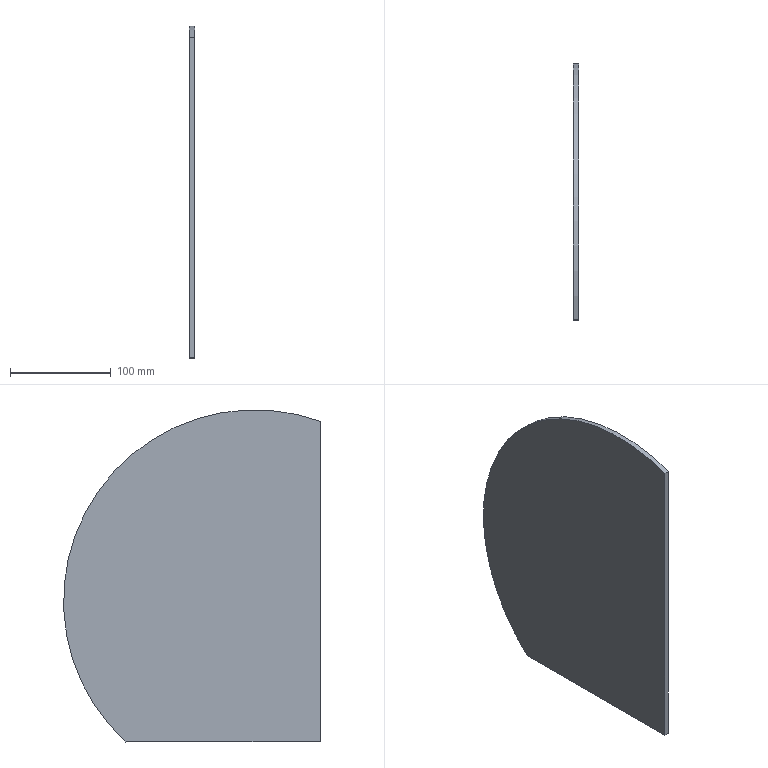Part | STEP file | 09-13 Outer base plate 2 | 1 solid | 5 faces | box 5 x 255 x 330 mm | volume 367508 mm3 | plane 4 | cylinder 1 | commonest cylinder face diameters 380 x1
STEP:
#1=CARTESIAN_POINT('',(0.,0.,0.));
#2=DIRECTION('',(0.,0.,1.));
#3=DIRECTION('',(1.,0.,0.));
#4=AXIS2_PLACEMENT_3D('',#1,#2,#3);
#5=CARTESIAN_POINT('',(5.,188.452,-490.));
#6=VERTEX_POINT('',#5);
#7=CARTESIAN_POINT('',(5.,-5.,-171.464));
#8=VERTEX_POINT('',#7);
#9=CARTESIAN_POINT('',(5.,60.,-350.));
#10=DIRECTION('',(1.,0.,0.));
#11=DIRECTION('',(0.,-1.,0.));
#12=AXIS2_PLACEMENT_3D('',#9,#10,#11);
#13=CIRCLE('',#12,190.);
#14=CARTESIAN_POINT('',(5.,60.,-350.));
#15=DIRECTION('',(-1.,0.,0.));
#16=DIRECTION('',(0.,-1.,0.));
#17=AXIS2_PLACEMENT_3D('',#14,#15,#16);
#18=CYLINDRICAL_SURFACE('',#17,190.);
#19=CARTESIAN_POINT('',(6.283,0.));
#20=DIRECTION('',(-1.,0.));
#21=VECTOR('',#20,1.);
#22=LINE('',#19,#21);
#23=(GEOMETRIC_REPRESENTATION_CONTEXT(2)PARAMETRIC_REPRESENTATION_CONTEXT()REPRESENTATION_CONTEXT('',''));
#24=DEFINITIONAL_REPRESENTATION('',(#22),#23);
#25=PCURVE('',#18,#24);
#26=CARTESIAN_POINT('',(5.,-5.,-158.02));
#27=DIRECTION('',(1.,0.,0.));
#28=DIRECTION('',(0.,0.,-1.));
#29=AXIS2_PLACEMENT_3D('',#26,#27,#28);
#30=PLANE('',#29);
#31=CARTESIAN_POINT('',(191.98,65.));
#32=DIRECTION('',(0.,-1.));
#33=AXIS2_PLACEMENT_2D('',#31,#32);
#34=CIRCLE('',#33,190.);
#35=(GEOMETRIC_REPRESENTATION_CONTEXT(2)PARAMETRIC_REPRESENTATION_CONTEXT()REPRESENTATION_CONTEXT('',''));
#36=DEFINITIONAL_REPRESENTATION('',(#34),#35);
#37=PCURVE('',#30,#36);
#38=SURFACE_CURVE('',#13,(#25,#37),.PCURVE_S1.);
#39=EDGE_CURVE('',#6,#8,#38,.T.);
#40=ORIENTED_EDGE('',*,*,#39,.F.);
#41=CARTESIAN_POINT('',(0.,188.452,-490.));
#42=VERTEX_POINT('',#41);
#43=CARTESIAN_POINT('',(2.5,188.452,-490.));
#44=DIRECTION('',(1.,0.,0.));
#45=VECTOR('',#44,1.);
#46=LINE('',#43,#45);
#47=CARTESIAN_POINT('',(3.97,2.5));
#48=DIRECTION('',(0.,-1.));
#49=VECTOR('',#48,1.);
#50=LINE('',#47,#49);
#51=(GEOMETRIC_REPRESENTATION_CONTEXT(2)PARAMETRIC_REPRESENTATION_CONTEXT()REPRESENTATION_CONTEXT('',''));
#52=DEFINITIONAL_REPRESENTATION('',(#50),#51);
#53=PCURVE('',#18,#52);
#54=CARTESIAN_POINT('',(0.,188.452,-490.));
#55=DIRECTION('',(0.,0.,1.));
#56=DIRECTION('',(0.,-1.,0.));
#57=AXIS2_PLACEMENT_3D('',#54,#55,#56);
#58=PLANE('',#57);
#59=CARTESIAN_POINT('',(0.000000061,2.5));
#60=DIRECTION('',(0.,1.));
#61=VECTOR('',#60,1.);
#62=LINE('',#59,#61);
#63=(GEOMETRIC_REPRESENTATION_CONTEXT(2)PARAMETRIC_REPRESENTATION_CONTEXT()REPRESENTATION_CONTEXT('',''));
#64=DEFINITIONAL_REPRESENTATION('',(#62),#63);
#65=PCURVE('',#58,#64);
#66=SURFACE_CURVE('',#46,(#53,#65),.PCURVE_S1.);
#67=EDGE_CURVE('',#42,#6,#66,.T.);
#68=ORIENTED_EDGE('',*,*,#67,.F.);
#69=CARTESIAN_POINT('',(0.,-5.,-171.464));
#70=VERTEX_POINT('',#69);
#71=CARTESIAN_POINT('',(0.,60.,-350.));
#72=DIRECTION('',(-1.,0.,0.));
#73=DIRECTION('',(0.,-1.,0.));
#74=AXIS2_PLACEMENT_3D('',#71,#72,#73);
#75=CIRCLE('',#74,190.);
#76=CARTESIAN_POINT('',(0.,5.));
#77=DIRECTION('',(1.,0.));
#78=VECTOR('',#77,1.);
#79=LINE('',#76,#78);
#80=(GEOMETRIC_REPRESENTATION_CONTEXT(2)PARAMETRIC_REPRESENTATION_CONTEXT()REPRESENTATION_CONTEXT('',''));
#81=DEFINITIONAL_REPRESENTATION('',(#79),#80);
#82=PCURVE('',#18,#81);
#83=CARTESIAN_POINT('',(0.,-5.,-158.02));
#84=DIRECTION('',(1.,0.,0.));
#85=DIRECTION('',(0.,0.,-1.));
#86=AXIS2_PLACEMENT_3D('',#83,#84,#85);
#87=PLANE('',#86);
#88=CARTESIAN_POINT('',(191.98,-125.));
#89=CARTESIAN_POINT('',(-137.11,-125.));
#90=CARTESIAN_POINT('',(27.435,160.));
#91=CARTESIAN_POINT('',(191.98,445.));
#92=CARTESIAN_POINT('',(356.525,160.));
#93=CARTESIAN_POINT('',(521.07,-125.));
#94=CARTESIAN_POINT('',(191.98,-125.));
#95=(BOUNDED_CURVE()B_SPLINE_CURVE(2,(#88,#89,#90,#91,#92,#93,#94),.UNSPECIFIED.,.T.,.F.)B_SPLINE_CURVE_WITH_KNOTS((1,2,2,2,2,1),(-2.094,0.,2.094,4.189,6.283,8.378),.UNSPECIFIED.)CURVE()GEOMETRIC_REPRESENTATION_ITEM()RATIONAL_B_SPLINE_CURVE((1.,0.5,1.,0.5,1.,0.5,1.))REPRESENTATION_ITEM(''));
#96=(GEOMETRIC_REPRESENTATION_CONTEXT(2)PARAMETRIC_REPRESENTATION_CONTEXT()REPRESENTATION_CONTEXT('',''));
#97=DEFINITIONAL_REPRESENTATION('',(#95),#96);
#98=PCURVE('',#87,#97);
#99=SURFACE_CURVE('',#75,(#82,#98),.PCURVE_S1.);
#100=EDGE_CURVE('',#70,#42,#99,.T.);
#101=ORIENTED_EDGE('',*,*,#100,.F.);
#102=CARTESIAN_POINT('',(2.5,-5.,-171.464));
#103=DIRECTION('',(-1.,0.,0.));
#104=VECTOR('',#103,1.);
#105=LINE('',#102,#104);
#106=CARTESIAN_POINT('',(1.222,2.5));
#107=DIRECTION('',(0.,1.));
#108=VECTOR('',#107,1.);
#109=LINE('',#106,#108);
#110=(GEOMETRIC_REPRESENTATION_CONTEXT(2)PARAMETRIC_REPRESENTATION_CONTEXT()REPRESENTATION_CONTEXT('',''));
#111=DEFINITIONAL_REPRESENTATION('',(#109),#110);
#112=PCURVE('',#18,#111);
#113=CARTESIAN_POINT('',(0.,-5.,-490.));
#114=DIRECTION('',(0.,1.,0.));
#115=DIRECTION('',(0.,0.,1.));
#116=AXIS2_PLACEMENT_3D('',#113,#114,#115);
#117=PLANE('',#116);
#118=CARTESIAN_POINT('',(318.536,2.5));
#119=DIRECTION('',(0.,-1.));
#120=VECTOR('',#119,1.);
#121=LINE('',#118,#120);
#122=(GEOMETRIC_REPRESENTATION_CONTEXT(2)PARAMETRIC_REPRESENTATION_CONTEXT()REPRESENTATION_CONTEXT('',''));
#123=DEFINITIONAL_REPRESENTATION('',(#121),#122);
#124=PCURVE('',#117,#123);
#125=SURFACE_CURVE('',#105,(#112,#124),.PCURVE_S1.);
#126=EDGE_CURVE('',#8,#70,#125,.T.);
#127=ORIENTED_EDGE('',*,*,#126,.F.);
#128=EDGE_LOOP('',(#40,#68,#101,#127));
#129=FACE_BOUND('',#128,.T.);
#130=ADVANCED_FACE('',(#129),#18,.T.);
#131=CARTESIAN_POINT('',(5.,-5.,-490.));
#132=VERTEX_POINT('',#131);
#133=CARTESIAN_POINT('',(5.,-5.,-324.01));
#134=DIRECTION('',(0.,0.,-1.));
#135=VECTOR('',#134,1.);
#136=LINE('',#133,#135);
#137=CARTESIAN_POINT('',(165.99,0.));
#138=DIRECTION('',(1.,0.));
#139=VECTOR('',#138,1.);
#140=LINE('',#137,#139);
#141=(GEOMETRIC_REPRESENTATION_CONTEXT(2)PARAMETRIC_REPRESENTATION_CONTEXT()REPRESENTATION_CONTEXT('',''));
#142=DEFINITIONAL_REPRESENTATION('',(#140),#141);
#143=PCURVE('',#30,#142);
#144=CARTESIAN_POINT('',(165.99,5.));
#145=DIRECTION('',(-1.,0.));
#146=VECTOR('',#145,1.);
#147=LINE('',#144,#146);
#148=(GEOMETRIC_REPRESENTATION_CONTEXT(2)PARAMETRIC_REPRESENTATION_CONTEXT()REPRESENTATION_CONTEXT('',''));
#149=DEFINITIONAL_REPRESENTATION('',(#147),#148);
#150=PCURVE('',#117,#149);
#151=SURFACE_CURVE('',#136,(#143,#150),.PCURVE_S1.);
#152=EDGE_CURVE('',#8,#132,#151,.T.);
#153=ORIENTED_EDGE('',*,*,#152,.T.);
#154=CARTESIAN_POINT('',(5.,123.265,-490.));
#155=DIRECTION('',(0.,1.,0.));
#156=VECTOR('',#155,1.);
#157=LINE('',#154,#156);
#158=CARTESIAN_POINT('',(331.98,128.265));
#159=DIRECTION('',(0.,1.));
#160=VECTOR('',#159,1.);
#161=LINE('',#158,#160);
#162=(GEOMETRIC_REPRESENTATION_CONTEXT(2)PARAMETRIC_REPRESENTATION_CONTEXT()REPRESENTATION_CONTEXT('',''));
#163=DEFINITIONAL_REPRESENTATION('',(#161),#162);
#164=PCURVE('',#30,#163);
#165=CARTESIAN_POINT('',(65.187,5.));
#166=DIRECTION('',(-1.,0.));
#167=VECTOR('',#166,1.);
#168=LINE('',#165,#167);
#169=(GEOMETRIC_REPRESENTATION_CONTEXT(2)PARAMETRIC_REPRESENTATION_CONTEXT()REPRESENTATION_CONTEXT('',''));
#170=DEFINITIONAL_REPRESENTATION('',(#168),#169);
#171=PCURVE('',#58,#170);
#172=SURFACE_CURVE('',#157,(#164,#171),.PCURVE_S1.);
#173=EDGE_CURVE('',#132,#6,#172,.T.);
#174=ORIENTED_EDGE('',*,*,#173,.T.);
#175=ORIENTED_EDGE('',*,*,#39,.T.);
#176=EDGE_LOOP('',(#153,#174,#175));
#177=FACE_BOUND('',#176,.T.);
#178=ADVANCED_FACE('',(#177),#30,.T.);
#179=CARTESIAN_POINT('',(0.,-5.,-490.));
#180=VERTEX_POINT('',#179);
#181=CARTESIAN_POINT('',(0.,123.265,-490.));
#182=DIRECTION('',(0.,1.,0.));
#183=VECTOR('',#182,1.);
#184=LINE('',#181,#183);
#185=CARTESIAN_POINT('',(331.98,128.265));
#186=DIRECTION('',(0.,1.));
#187=VECTOR('',#186,1.);
#188=LINE('',#185,#187);
#189=(GEOMETRIC_REPRESENTATION_CONTEXT(2)PARAMETRIC_REPRESENTATION_CONTEXT()REPRESENTATION_CONTEXT('',''));
#190=DEFINITIONAL_REPRESENTATION('',(#188),#189);
#191=PCURVE('',#87,#190);
#192=CARTESIAN_POINT('',(65.187,0.));
#193=DIRECTION('',(-1.,0.));
#194=VECTOR('',#193,1.);
#195=LINE('',#192,#194);
#196=(GEOMETRIC_REPRESENTATION_CONTEXT(2)PARAMETRIC_REPRESENTATION_CONTEXT()REPRESENTATION_CONTEXT('',''));
#197=DEFINITIONAL_REPRESENTATION('',(#195),#196);
#198=PCURVE('',#58,#197);
#199=SURFACE_CURVE('',#184,(#191,#198),.PCURVE_S1.);
#200=EDGE_CURVE('',#180,#42,#199,.T.);
#201=ORIENTED_EDGE('',*,*,#200,.F.);
#202=CARTESIAN_POINT('',(0.,-5.,-324.01));
#203=DIRECTION('',(0.,0.,-1.));
#204=VECTOR('',#203,1.);
#205=LINE('',#202,#204);
#206=CARTESIAN_POINT('',(165.99,0.));
#207=DIRECTION('',(1.,0.));
#208=VECTOR('',#207,1.);
#209=LINE('',#206,#208);
#210=(GEOMETRIC_REPRESENTATION_CONTEXT(2)PARAMETRIC_REPRESENTATION_CONTEXT()REPRESENTATION_CONTEXT('',''));
#211=DEFINITIONAL_REPRESENTATION('',(#209),#210);
#212=PCURVE('',#87,#211);
#213=CARTESIAN_POINT('',(165.99,0.));
#214=DIRECTION('',(-1.,0.));
#215=VECTOR('',#214,1.);
#216=LINE('',#213,#215);
#217=(GEOMETRIC_REPRESENTATION_CONTEXT(2)PARAMETRIC_REPRESENTATION_CONTEXT()REPRESENTATION_CONTEXT('',''));
#218=DEFINITIONAL_REPRESENTATION('',(#216),#217);
#219=PCURVE('',#117,#218);
#220=SURFACE_CURVE('',#205,(#212,#219),.PCURVE_S1.);
#221=EDGE_CURVE('',#70,#180,#220,.T.);
#222=ORIENTED_EDGE('',*,*,#221,.F.);
#223=ORIENTED_EDGE('',*,*,#100,.T.);
#224=EDGE_LOOP('',(#201,#222,#223));
#225=FACE_BOUND('',#224,.T.);
#226=ADVANCED_FACE('',(#225),#87,.F.);
#227=CARTESIAN_POINT('',(2.5,-5.,-490.));
#228=DIRECTION('',(-1.,0.,0.));
#229=VECTOR('',#228,1.);
#230=LINE('',#227,#229);
#231=CARTESIAN_POINT('',(0.,2.5));
#232=DIRECTION('',(0.,-1.));
#233=VECTOR('',#232,1.);
#234=LINE('',#231,#233);
#235=(GEOMETRIC_REPRESENTATION_CONTEXT(2)PARAMETRIC_REPRESENTATION_CONTEXT()REPRESENTATION_CONTEXT('',''));
#236=DEFINITIONAL_REPRESENTATION('',(#234),#235);
#237=PCURVE('',#117,#236);
#238=CARTESIAN_POINT('',(193.452,2.5));
#239=DIRECTION('',(0.,-1.));
#240=VECTOR('',#239,1.);
#241=LINE('',#238,#240);
#242=(GEOMETRIC_REPRESENTATION_CONTEXT(2)PARAMETRIC_REPRESENTATION_CONTEXT()REPRESENTATION_CONTEXT('',''));
#243=DEFINITIONAL_REPRESENTATION('',(#241),#242);
#244=PCURVE('',#58,#243);
#245=SURFACE_CURVE('',#230,(#237,#244),.PCURVE_S1.);
#246=EDGE_CURVE('',#132,#180,#245,.T.);
#247=ORIENTED_EDGE('',*,*,#246,.F.);
#248=ORIENTED_EDGE('',*,*,#152,.F.);
#249=ORIENTED_EDGE('',*,*,#126,.T.);
#250=ORIENTED_EDGE('',*,*,#221,.T.);
#251=EDGE_LOOP('',(#247,#248,#249,#250));
#252=FACE_BOUND('',#251,.T.);
#253=ADVANCED_FACE('',(#252),#117,.F.);
#254=ORIENTED_EDGE('',*,*,#67,.T.);
#255=ORIENTED_EDGE('',*,*,#173,.F.);
#256=ORIENTED_EDGE('',*,*,#246,.T.);
#257=ORIENTED_EDGE('',*,*,#200,.T.);
#258=EDGE_LOOP('',(#254,#255,#256,#257));
#259=FACE_BOUND('',#258,.T.);
#260=ADVANCED_FACE('',(#259),#58,.F.);
#261=CLOSED_SHELL('',(#130,#178,#226,#253,#260));
#262=MANIFOLD_SOLID_BREP('',#261);
#263=(LENGTH_UNIT()NAMED_UNIT(*)SI_UNIT(.MILLI.,.METRE.));
#264=UNCERTAINTY_MEASURE_WITH_UNIT(LENGTH_MEASURE(0.0000001),#263,'','');
#265=(NAMED_UNIT(*)PLANE_ANGLE_UNIT()SI_UNIT($,.RADIAN.));
#266=(NAMED_UNIT(*)SI_UNIT($,.STERADIAN.)SOLID_ANGLE_UNIT());
#267=(GEOMETRIC_REPRESENTATION_CONTEXT(3)GLOBAL_UNCERTAINTY_ASSIGNED_CONTEXT((#264))GLOBAL_UNIT_ASSIGNED_CONTEXT((#263,#265,#266))REPRESENTATION_CONTEXT('',''));
#268=ADVANCED_BREP_SHAPE_REPRESENTATION('',(#4,#262),#267);